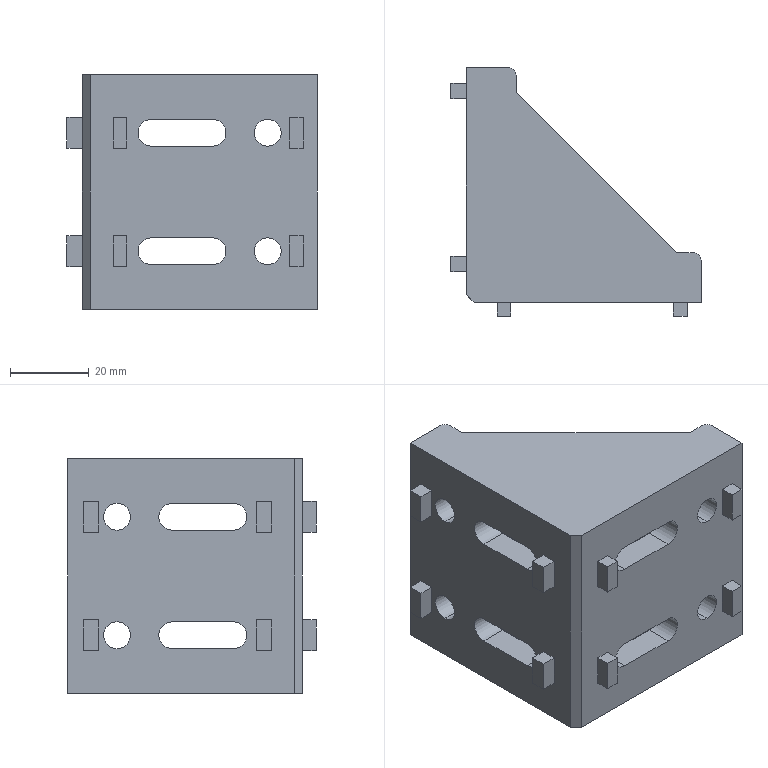Part | NX | features BREP 1 | 1 solid | 85 faces | box 63.4 x 63 x 59.5 mm | volume 51932 mm3 | plane 65 | cylinder 20 | commonest cylinder face diameters 6.8 x16 4 x4